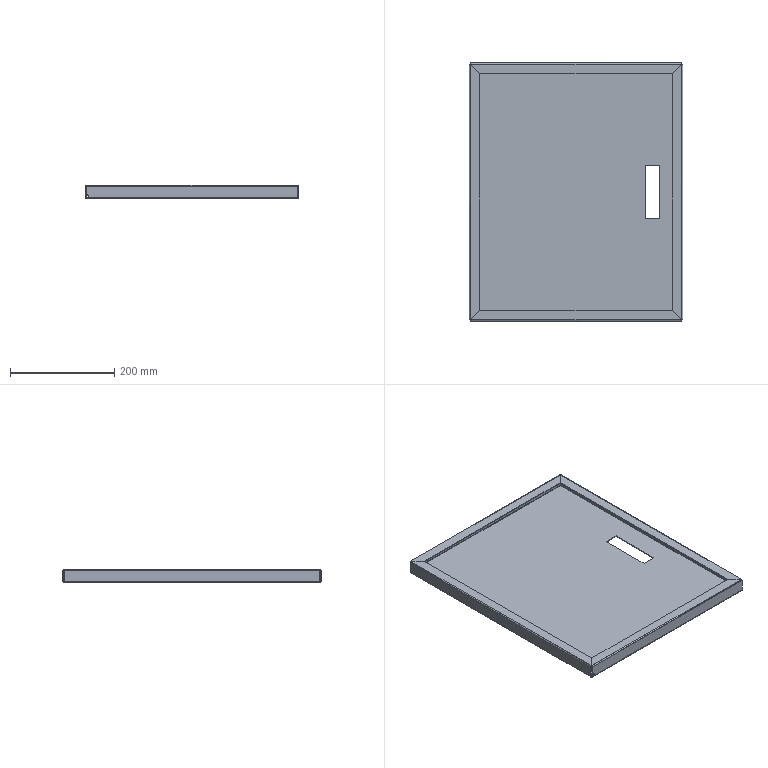Part | SolidWorks | features MirrorStock 1 | 1 solid | 78 faces | box 411 x 496 x 26.5 mm | volume 413789 mm3 | plane 42 | cylinder 20 | spline 16 | commonest cylinder face diameters 1 x8 4 x8 5 x4